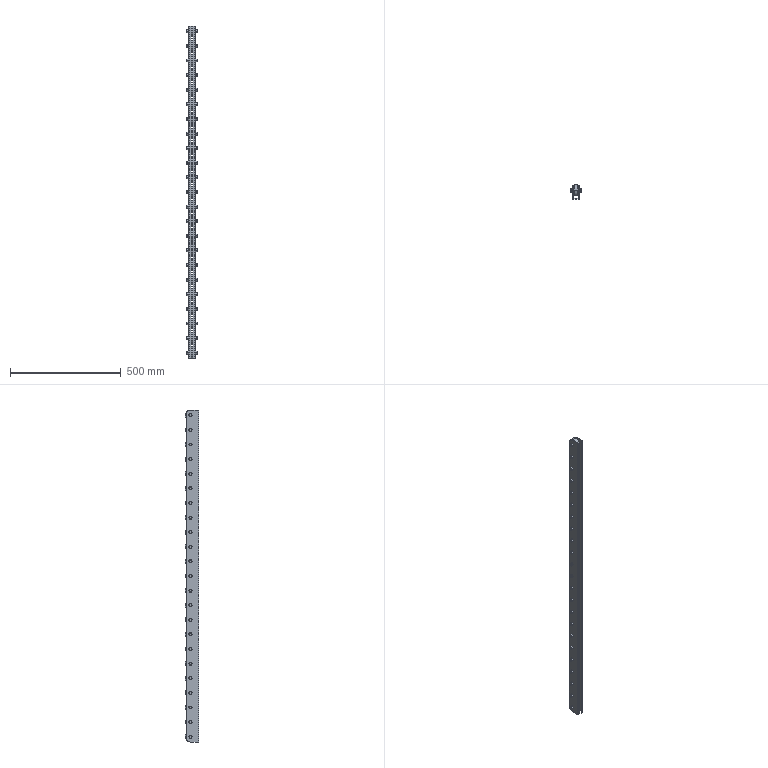Part | STEP file | Flow rail_default<machined> | 48 solids | 1500 faces | box 46 x 62.5 x 1500 mm | volume 1123340 mm3 | cylinder 610 | plane 522 | cone 276 | torus 92 | commonest cylinder face diameters 15 x276 8 x138 12 x92 8.2 x50 48 x46 40 x4